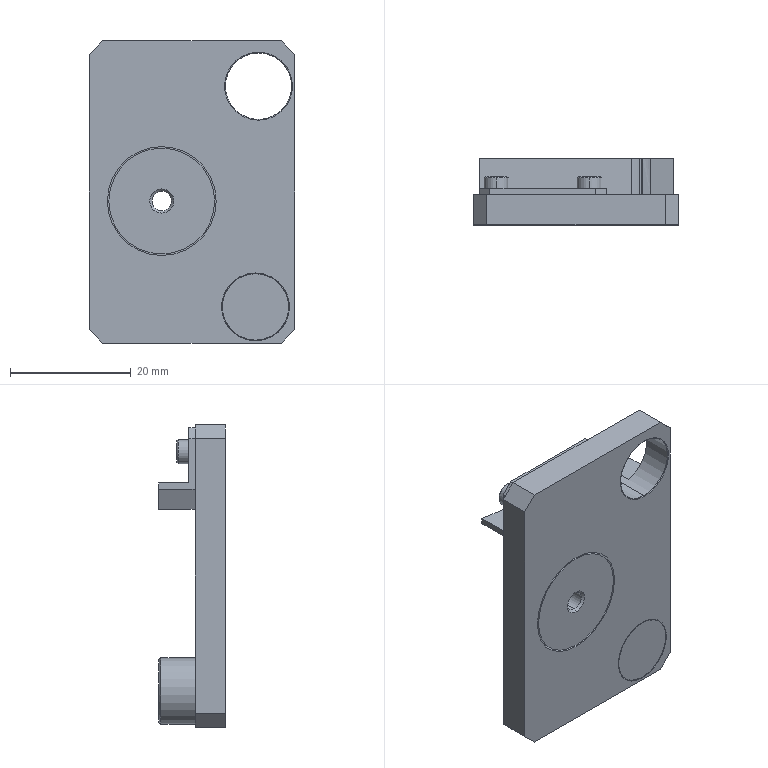Part | STEP file | b_SECWK14 | 1 solid | 92 faces | box 34 x 11 x 50 mm | volume 8847 mm3 | plane 48 | cylinder 28 | cone 10 | torus 6 | commonest cylinder face diameters 11 x6 4 x4 11.088 x4 17.5 x4 18 x4 3.242 x2